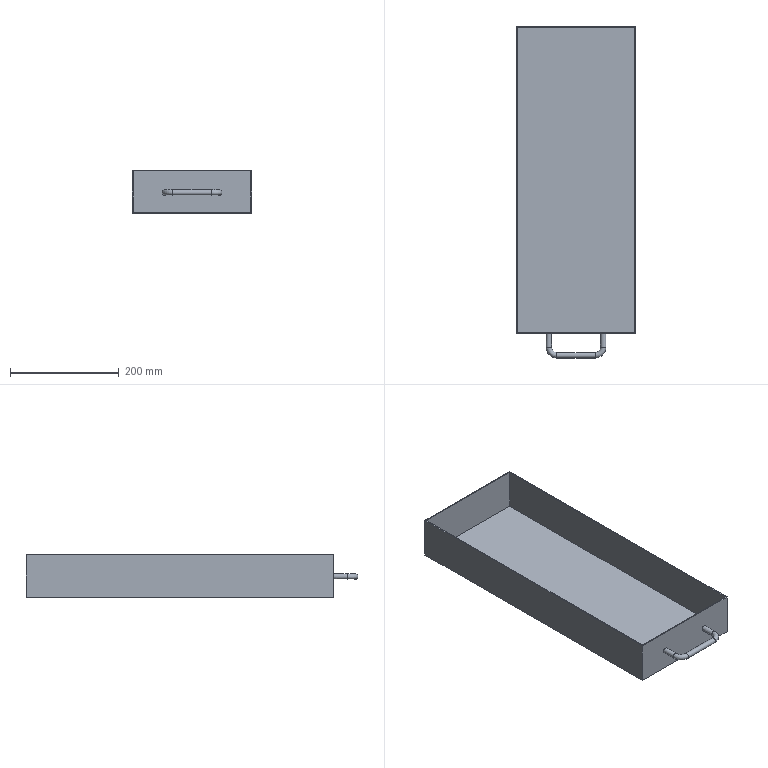Part | NX | features solid 2 | 1 solid | 16 faces | box 220 x 610 x 78 mm | volume 499150 mm3 | plane 11 | cylinder 3 | torus 2 | commonest cylinder face diameters 10 x3
STEP:
#1=CARTESIAN_POINT('',(425.,-410.,-285.));
#2=VERTEX_POINT('',#1);
#3=CARTESIAN_POINT('',(425.,-410.,-280.));
#4=DIRECTION('',(0.,-1.,0.));
#5=DIRECTION('',(0.,0.,-1.));
#6=AXIS2_PLACEMENT_3D('',#3,#4,#5);
#7=CIRCLE('',#6,5.);
#8=EDGE_CURVE('',#2,#2,#7,.T.);
#9=ORIENTED_EDGE('',*,*,#8,.F.);
#10=EDGE_LOOP('',(#9));
#11=FACE_BOUND('',#10,.T.);
#12=CARTESIAN_POINT('',(365.,-410.,-240.));
#13=VERTEX_POINT('',#12);
#14=CARTESIAN_POINT('',(585.,-410.,-240.));
#15=VERTEX_POINT('',#14);
#16=CARTESIAN_POINT('',(-350.,-410.,-240.));
#17=DIRECTION('',(1.,0.,0.));
#18=VECTOR('',#17,1000.);
#19=LINE('',#16,#18);
#20=EDGE_CURVE('',#13,#15,#19,.T.);
#21=ORIENTED_EDGE('',*,*,#20,.F.);
#22=CARTESIAN_POINT('',(365.,-410.,-318.));
#23=VERTEX_POINT('',#22);
#24=CARTESIAN_POINT('',(365.,-410.,0.));
#25=DIRECTION('',(0.,0.,1.));
#26=VECTOR('',#25,1000.);
#27=LINE('',#24,#26);
#28=EDGE_CURVE('',#23,#13,#27,.T.);
#29=ORIENTED_EDGE('',*,*,#28,.F.);
#30=CARTESIAN_POINT('',(585.,-410.,-318.));
#31=VERTEX_POINT('',#30);
#32=CARTESIAN_POINT('',(-350.,-410.,-318.));
#33=DIRECTION('',(-1.,0.,0.));
#34=VECTOR('',#33,1000.);
#35=LINE('',#32,#34);
#36=EDGE_CURVE('',#23,#31,#35,.F.);
#37=ORIENTED_EDGE('',*,*,#36,.T.);
#38=CARTESIAN_POINT('',(585.,-410.,0.));
#39=DIRECTION('',(0.,0.,1.));
#40=VECTOR('',#39,1000.);
#41=LINE('',#38,#40);
#42=EDGE_CURVE('',#31,#15,#41,.T.);
#43=ORIENTED_EDGE('',*,*,#42,.T.);
#44=EDGE_LOOP('',(#21,#29,#37,#43));
#45=FACE_BOUND('',#44,.T.);
#46=CARTESIAN_POINT('',(520.,-410.,-280.));
#47=VERTEX_POINT('',#46);
#48=CARTESIAN_POINT('',(525.,-410.,-280.));
#49=DIRECTION('',(0.,-1.,0.));
#50=DIRECTION('',(-1.,0.,0.));
#51=AXIS2_PLACEMENT_3D('',#48,#49,#50);
#52=CIRCLE('',#51,5.);
#53=EDGE_CURVE('',#47,#47,#52,.T.);
#54=ORIENTED_EDGE('',*,*,#53,.F.);
#55=EDGE_LOOP('',(#54));
#56=FACE_BOUND('',#55,.T.);
#57=CARTESIAN_POINT('',(360.,-410.,0.));
#58=DIRECTION('',(0.,-1.,0.));
#59=DIRECTION('',(0.,0.,-1.));
#60=AXIS2_PLACEMENT_3D('',#57,#58,#59);
#61=PLANE('',#60);
#62=ADVANCED_FACE('',(#11,#45,#56),#61,.T.);
#63=CARTESIAN_POINT('',(365.,155.,-240.));
#64=VERTEX_POINT('',#63);
#65=CARTESIAN_POINT('',(365.,105.,-240.));
#66=DIRECTION('',(0.,-1.,0.));
#67=VECTOR('',#66,1000.);
#68=LINE('',#65,#67);
#69=EDGE_CURVE('',#64,#13,#68,.T.);
#70=ORIENTED_EDGE('',*,*,#69,.F.);
#71=CARTESIAN_POINT('',(365.,155.,-318.));
#72=VERTEX_POINT('',#71);
#73=CARTESIAN_POINT('',(365.,155.,0.));
#74=DIRECTION('',(0.,0.,1.));
#75=VECTOR('',#74,1000.);
#76=LINE('',#73,#75);
#77=EDGE_CURVE('',#72,#64,#76,.T.);
#78=ORIENTED_EDGE('',*,*,#77,.F.);
#79=CARTESIAN_POINT('',(365.,-70.,-318.));
#80=DIRECTION('',(0.,1.,0.));
#81=VECTOR('',#80,1000.);
#82=LINE('',#79,#81);
#83=EDGE_CURVE('',#72,#23,#82,.F.);
#84=ORIENTED_EDGE('',*,*,#83,.T.);
#85=ORIENTED_EDGE('',*,*,#28,.T.);
#86=EDGE_LOOP('',(#70,#78,#84,#85));
#87=FACE_BOUND('',#86,.T.);
#88=CARTESIAN_POINT('',(365.,175.,0.));
#89=DIRECTION('',(-1.,0.,0.));
#90=DIRECTION('',(0.,0.,1.));
#91=AXIS2_PLACEMENT_3D('',#88,#89,#90);
#92=PLANE('',#91);
#93=ADVANCED_FACE('',(#87),#92,.T.);
#94=CARTESIAN_POINT('',(585.,155.,-240.));
#95=VERTEX_POINT('',#94);
#96=CARTESIAN_POINT('',(585.,105.,-240.));
#97=DIRECTION('',(0.,1.,0.));
#98=VECTOR('',#97,1000.);
#99=LINE('',#96,#98);
#100=EDGE_CURVE('',#15,#95,#99,.T.);
#101=ORIENTED_EDGE('',*,*,#100,.F.);
#102=ORIENTED_EDGE('',*,*,#42,.F.);
#103=CARTESIAN_POINT('',(585.,155.,-318.));
#104=VERTEX_POINT('',#103);
#105=CARTESIAN_POINT('',(585.,-70.,-318.));
#106=DIRECTION('',(0.,-1.,0.));
#107=VECTOR('',#106,1000.);
#108=LINE('',#105,#107);
#109=EDGE_CURVE('',#31,#104,#108,.F.);
#110=ORIENTED_EDGE('',*,*,#109,.T.);
#111=CARTESIAN_POINT('',(585.,155.,0.));
#112=DIRECTION('',(0.,0.,1.));
#113=VECTOR('',#112,1000.);
#114=LINE('',#111,#113);
#115=EDGE_CURVE('',#104,#95,#114,.T.);
#116=ORIENTED_EDGE('',*,*,#115,.T.);
#117=EDGE_LOOP('',(#101,#102,#110,#116));
#118=FACE_BOUND('',#117,.T.);
#119=CARTESIAN_POINT('',(585.,-460.,0.));
#120=DIRECTION('',(1.,0.,0.));
#121=DIRECTION('',(0.,0.,-1.));
#122=AXIS2_PLACEMENT_3D('',#119,#120,#121);
#123=PLANE('',#122);
#124=ADVANCED_FACE('',(#118),#123,.T.);
#125=CARTESIAN_POINT('',(-350.,155.,-240.));
#126=DIRECTION('',(-1.,0.,0.));
#127=VECTOR('',#126,1000.);
#128=LINE('',#125,#127);
#129=EDGE_CURVE('',#95,#64,#128,.T.);
#130=ORIENTED_EDGE('',*,*,#129,.F.);
#131=ORIENTED_EDGE('',*,*,#115,.F.);
#132=CARTESIAN_POINT('',(-350.,155.,-318.));
#133=DIRECTION('',(1.,0.,0.));
#134=VECTOR('',#133,1000.);
#135=LINE('',#132,#134);
#136=EDGE_CURVE('',#104,#72,#135,.F.);
#137=ORIENTED_EDGE('',*,*,#136,.T.);
#138=ORIENTED_EDGE('',*,*,#77,.T.);
#139=EDGE_LOOP('',(#130,#131,#137,#138));
#140=FACE_BOUND('',#139,.T.);
#141=CARTESIAN_POINT('',(585.,155.,0.));
#142=DIRECTION('',(0.,1.,0.));
#143=DIRECTION('',(0.,0.,1.));
#144=AXIS2_PLACEMENT_3D('',#141,#142,#143);
#145=PLANE('',#144);
#146=ADVANCED_FACE('',(#140),#145,.T.);
#147=ORIENTED_EDGE('',*,*,#83,.F.);
#148=ORIENTED_EDGE('',*,*,#136,.F.);
#149=ORIENTED_EDGE('',*,*,#109,.F.);
#150=ORIENTED_EDGE('',*,*,#36,.F.);
#151=EDGE_LOOP('',(#147,#148,#149,#150));
#152=FACE_BOUND('',#151,.T.);
#153=CARTESIAN_POINT('',(-350.,-70.,-318.));
#154=DIRECTION('',(0.,0.,-1.));
#155=DIRECTION('',(-1.,0.,0.));
#156=AXIS2_PLACEMENT_3D('',#153,#154,#155);
#157=PLANE('',#156);
#158=ADVANCED_FACE('',(#152),#157,.T.);
#159=CARTESIAN_POINT('',(367.,153.,-240.));
#160=VERTEX_POINT('',#159);
#161=CARTESIAN_POINT('',(367.,-408.,-240.));
#162=VERTEX_POINT('',#161);
#163=CARTESIAN_POINT('',(367.,105.,-240.));
#164=DIRECTION('',(0.,-1.,0.));
#165=VECTOR('',#164,1000.);
#166=LINE('',#163,#165);
#167=EDGE_CURVE('',#160,#162,#166,.T.);
#168=ORIENTED_EDGE('',*,*,#167,.F.);
#169=CARTESIAN_POINT('',(583.,153.,-240.));
#170=VERTEX_POINT('',#169);
#171=CARTESIAN_POINT('',(-350.,153.,-240.));
#172=DIRECTION('',(-1.,0.,0.));
#173=VECTOR('',#172,1000.);
#174=LINE('',#171,#173);
#175=EDGE_CURVE('',#170,#160,#174,.T.);
#176=ORIENTED_EDGE('',*,*,#175,.F.);
#177=CARTESIAN_POINT('',(583.,-408.,-240.));
#178=VERTEX_POINT('',#177);
#179=CARTESIAN_POINT('',(583.,105.,-240.));
#180=DIRECTION('',(0.,1.,0.));
#181=VECTOR('',#180,1000.);
#182=LINE('',#179,#181);
#183=EDGE_CURVE('',#178,#170,#182,.T.);
#184=ORIENTED_EDGE('',*,*,#183,.F.);
#185=CARTESIAN_POINT('',(-350.,-408.,-240.));
#186=DIRECTION('',(1.,0.,0.));
#187=VECTOR('',#186,1000.);
#188=LINE('',#185,#187);
#189=EDGE_CURVE('',#162,#178,#188,.T.);
#190=ORIENTED_EDGE('',*,*,#189,.F.);
#191=EDGE_LOOP('',(#168,#176,#184,#190));
#192=FACE_BOUND('',#191,.T.);
#193=ORIENTED_EDGE('',*,*,#69,.T.);
#194=ORIENTED_EDGE('',*,*,#20,.T.);
#195=ORIENTED_EDGE('',*,*,#100,.T.);
#196=ORIENTED_EDGE('',*,*,#129,.T.);
#197=EDGE_LOOP('',(#193,#194,#195,#196));
#198=FACE_BOUND('',#197,.T.);
#199=CARTESIAN_POINT('',(-350.,105.,-240.));
#200=DIRECTION('',(0.,0.,1.));
#201=DIRECTION('',(1.,0.,0.));
#202=AXIS2_PLACEMENT_3D('',#199,#200,#201);
#203=PLANE('',#202);
#204=ADVANCED_FACE('',(#192,#198),#203,.T.);
#205=ORIENTED_EDGE('',*,*,#167,.T.);
#206=CARTESIAN_POINT('',(367.,-408.,-316.));
#207=VERTEX_POINT('',#206);
#208=CARTESIAN_POINT('',(367.,-408.,0.));
#209=DIRECTION('',(0.,0.,1.));
#210=VECTOR('',#209,1000.);
#211=LINE('',#208,#210);
#212=EDGE_CURVE('',#207,#162,#211,.T.);
#213=ORIENTED_EDGE('',*,*,#212,.F.);
#214=CARTESIAN_POINT('',(367.,153.,-316.));
#215=VERTEX_POINT('',#214);
#216=CARTESIAN_POINT('',(367.,-70.,-316.));
#217=DIRECTION('',(0.,1.,0.));
#218=VECTOR('',#217,1000.);
#219=LINE('',#216,#218);
#220=EDGE_CURVE('',#215,#207,#219,.F.);
#221=ORIENTED_EDGE('',*,*,#220,.F.);
#222=CARTESIAN_POINT('',(367.,153.,0.));
#223=DIRECTION('',(0.,0.,1.));
#224=VECTOR('',#223,1000.);
#225=LINE('',#222,#224);
#226=EDGE_CURVE('',#215,#160,#225,.T.);
#227=ORIENTED_EDGE('',*,*,#226,.T.);
#228=EDGE_LOOP('',(#205,#213,#221,#227));
#229=FACE_BOUND('',#228,.T.);
#230=CARTESIAN_POINT('',(367.,175.,0.));
#231=DIRECTION('',(-1.,0.,0.));
#232=DIRECTION('',(0.,0.,1.));
#233=AXIS2_PLACEMENT_3D('',#230,#231,#232);
#234=PLANE('',#233);
#235=ADVANCED_FACE('',(#229),#234,.F.);
#236=ORIENTED_EDGE('',*,*,#189,.T.);
#237=CARTESIAN_POINT('',(583.,-408.,-316.));
#238=VERTEX_POINT('',#237);
#239=CARTESIAN_POINT('',(583.,-408.,0.));
#240=DIRECTION('',(0.,0.,1.));
#241=VECTOR('',#240,1000.);
#242=LINE('',#239,#241);
#243=EDGE_CURVE('',#238,#178,#242,.T.);
#244=ORIENTED_EDGE('',*,*,#243,.F.);
#245=CARTESIAN_POINT('',(-350.,-408.,-316.));
#246=DIRECTION('',(-1.,0.,0.));
#247=VECTOR('',#246,1000.);
#248=LINE('',#245,#247);
#249=EDGE_CURVE('',#207,#238,#248,.F.);
#250=ORIENTED_EDGE('',*,*,#249,.F.);
#251=ORIENTED_EDGE('',*,*,#212,.T.);
#252=EDGE_LOOP('',(#236,#244,#250,#251));
#253=FACE_BOUND('',#252,.T.);
#254=CARTESIAN_POINT('',(360.,-408.,0.));
#255=DIRECTION('',(0.,-1.,0.));
#256=DIRECTION('',(0.,0.,-1.));
#257=AXIS2_PLACEMENT_3D('',#254,#255,#256);
#258=PLANE('',#257);
#259=ADVANCED_FACE('',(#253),#258,.F.);
#260=ORIENTED_EDGE('',*,*,#183,.T.);
#261=CARTESIAN_POINT('',(583.,153.,-316.));
#262=VERTEX_POINT('',#261);
#263=CARTESIAN_POINT('',(583.,153.,0.));
#264=DIRECTION('',(0.,0.,1.));
#265=VECTOR('',#264,1000.);
#266=LINE('',#263,#265);
#267=EDGE_CURVE('',#262,#170,#266,.T.);
#268=ORIENTED_EDGE('',*,*,#267,.F.);
#269=CARTESIAN_POINT('',(583.,-70.,-316.));
#270=DIRECTION('',(0.,-1.,0.));
#271=VECTOR('',#270,1000.);
#272=LINE('',#269,#271);
#273=EDGE_CURVE('',#238,#262,#272,.F.);
#274=ORIENTED_EDGE('',*,*,#273,.F.);
#275=ORIENTED_EDGE('',*,*,#243,.T.);
#276=EDGE_LOOP('',(#260,#268,#274,#275));
#277=FACE_BOUND('',#276,.T.);
#278=CARTESIAN_POINT('',(583.,-460.,0.));
#279=DIRECTION('',(1.,0.,0.));
#280=DIRECTION('',(0.,0.,-1.));
#281=AXIS2_PLACEMENT_3D('',#278,#279,#280);
#282=PLANE('',#281);
#283=ADVANCED_FACE('',(#277),#282,.F.);
#284=ORIENTED_EDGE('',*,*,#175,.T.);
#285=ORIENTED_EDGE('',*,*,#226,.F.);
#286=CARTESIAN_POINT('',(-350.,153.,-316.));
#287=DIRECTION('',(1.,0.,0.));
#288=VECTOR('',#287,1000.);
#289=LINE('',#286,#288);
#290=EDGE_CURVE('',#262,#215,#289,.F.);
#291=ORIENTED_EDGE('',*,*,#290,.F.);
#292=ORIENTED_EDGE('',*,*,#267,.T.);
#293=EDGE_LOOP('',(#284,#285,#291,#292));
#294=FACE_BOUND('',#293,.T.);
#295=CARTESIAN_POINT('',(585.,153.,0.));
#296=DIRECTION('',(0.,1.,0.));
#297=DIRECTION('',(0.,0.,1.));
#298=AXIS2_PLACEMENT_3D('',#295,#296,#297);
#299=PLANE('',#298);
#300=ADVANCED_FACE('',(#294),#299,.F.);
#301=ORIENTED_EDGE('',*,*,#220,.T.);
#302=ORIENTED_EDGE('',*,*,#249,.T.);
#303=ORIENTED_EDGE('',*,*,#273,.T.);
#304=ORIENTED_EDGE('',*,*,#290,.T.);
#305=EDGE_LOOP('',(#301,#302,#303,#304));
#306=FACE_BOUND('',#305,.T.);
#307=CARTESIAN_POINT('',(-350.,-70.,-316.));
#308=DIRECTION('',(0.,0.,-1.));
#309=DIRECTION('',(-1.,0.,0.));
#310=AXIS2_PLACEMENT_3D('',#307,#308,#309);
#311=PLANE('',#310);
#312=ADVANCED_FACE('',(#306),#311,.F.);
#313=CARTESIAN_POINT('',(520.,-435.,-280.));
#314=VERTEX_POINT('',#313);
#315=CARTESIAN_POINT('',(525.,-435.,-280.));
#316=DIRECTION('',(0.,-1.,0.));
#317=DIRECTION('',(-1.,0.,0.));
#318=AXIS2_PLACEMENT_3D('',#315,#316,#317);
#319=CIRCLE('',#318,5.);
#320=EDGE_CURVE('',#314,#314,#319,.T.);
#321=ORIENTED_EDGE('',*,*,#320,.F.);
#322=EDGE_LOOP('',(#321));
#323=FACE_BOUND('',#322,.T.);
#324=ORIENTED_EDGE('',*,*,#53,.T.);
#325=EDGE_LOOP('',(#324));
#326=FACE_BOUND('',#325,.T.);
#327=CARTESIAN_POINT('',(525.,-435.,-280.));
#328=DIRECTION('',(0.,1.,0.));
#329=DIRECTION('',(0.,0.,1.));
#330=AXIS2_PLACEMENT_3D('',#327,#328,#329);
#331=CYLINDRICAL_SURFACE('',#330,5.);
#332=ADVANCED_FACE('',(#323,#326),#331,.T.);
#333=CARTESIAN_POINT('',(510.,-445.,-280.));
#334=VERTEX_POINT('',#333);
#335=CARTESIAN_POINT('',(510.,-450.,-280.));
#336=DIRECTION('',(-1.,0.,0.));
#337=DIRECTION('',(0.,1.,0.));
#338=AXIS2_PLACEMENT_3D('',#335,#336,#337);
#339=CIRCLE('',#338,5.);
#340=EDGE_CURVE('',#334,#334,#339,.T.);
#341=ORIENTED_EDGE('',*,*,#340,.F.);
#342=EDGE_LOOP('',(#341));
#343=FACE_BOUND('',#342,.T.);
#344=ORIENTED_EDGE('',*,*,#320,.T.);
#345=EDGE_LOOP('',(#344));
#346=FACE_BOUND('',#345,.T.);
#347=CARTESIAN_POINT('',(510.,-435.,-280.));
#348=DIRECTION('',(0.,0.,1.));
#349=DIRECTION('',(1.,0.,0.));
#350=AXIS2_PLACEMENT_3D('',#347,#348,#349);
#351=TOROIDAL_SURFACE('',#350,15.,5.);
#352=ADVANCED_FACE('',(#343,#346),#351,.T.);
#353=ORIENTED_EDGE('',*,*,#340,.T.);
#354=EDGE_LOOP('',(#353));
#355=FACE_BOUND('',#354,.T.);
#356=CARTESIAN_POINT('',(440.,-445.,-280.));
#357=VERTEX_POINT('',#356);
#358=CARTESIAN_POINT('',(440.,-450.,-280.));
#359=DIRECTION('',(-1.,0.,0.));
#360=DIRECTION('',(0.,1.,0.));
#361=AXIS2_PLACEMENT_3D('',#358,#359,#360);
#362=CIRCLE('',#361,5.);
#363=EDGE_CURVE('',#357,#357,#362,.T.);
#364=ORIENTED_EDGE('',*,*,#363,.F.);
#365=EDGE_LOOP('',(#364));
#366=FACE_BOUND('',#365,.T.);
#367=CARTESIAN_POINT('',(440.,-450.,-280.));
#368=DIRECTION('',(1.,0.,0.));
#369=DIRECTION('',(0.,0.,-1.));
#370=AXIS2_PLACEMENT_3D('',#367,#368,#369);
#371=CYLINDRICAL_SURFACE('',#370,5.);
#372=ADVANCED_FACE('',(#355,#366),#371,.T.);
#373=CARTESIAN_POINT('',(430.,-435.,-280.));
#374=VERTEX_POINT('',#373);
#375=CARTESIAN_POINT('',(425.,-435.,-280.));
#376=DIRECTION('',(0.,1.,0.));
#377=DIRECTION('',(1.,0.,0.));
#378=AXIS2_PLACEMENT_3D('',#375,#376,#377);
#379=CIRCLE('',#378,5.);
#380=EDGE_CURVE('',#374,#374,#379,.T.);
#381=ORIENTED_EDGE('',*,*,#380,.F.);
#382=EDGE_LOOP('',(#381));
#383=FACE_BOUND('',#382,.T.);
#384=ORIENTED_EDGE('',*,*,#363,.T.);
#385=EDGE_LOOP('',(#384));
#386=FACE_BOUND('',#385,.T.);
#387=CARTESIAN_POINT('',(440.,-435.,-280.));
#388=DIRECTION('',(0.,0.,1.));
#389=DIRECTION('',(1.,0.,0.));
#390=AXIS2_PLACEMENT_3D('',#387,#388,#389);
#391=TOROIDAL_SURFACE('',#390,15.,5.);
#392=ADVANCED_FACE('',(#383,#386),#391,.T.);
#393=ORIENTED_EDGE('',*,*,#380,.T.);
#394=EDGE_LOOP('',(#393));
#395=FACE_BOUND('',#394,.T.);
#396=ORIENTED_EDGE('',*,*,#8,.T.);
#397=EDGE_LOOP('',(#396));
#398=FACE_BOUND('',#397,.T.);
#399=CARTESIAN_POINT('',(425.,-435.,-280.));
#400=DIRECTION('',(0.,1.,0.));
#401=DIRECTION('',(0.,0.,1.));
#402=AXIS2_PLACEMENT_3D('',#399,#400,#401);
#403=CYLINDRICAL_SURFACE('',#402,5.);
#404=ADVANCED_FACE('',(#395,#398),#403,.T.);
#405=CLOSED_SHELL('',(#62,#93,#124,#146,#158,#204,#235,#259,#283,#300,#312,#332,#352,#372,#392,#404));
#406=MANIFOLD_SOLID_BREP('',#405);
#407=(LENGTH_UNIT()NAMED_UNIT(*)SI_UNIT(.MILLI.,.METRE.));
#408=UNCERTAINTY_MEASURE_WITH_UNIT(LENGTH_MEASURE(0.00001),#407,'','');
#409=(NAMED_UNIT(*)PLANE_ANGLE_UNIT()SI_UNIT($,.RADIAN.));
#410=(NAMED_UNIT(*)SI_UNIT($,.STERADIAN.)SOLID_ANGLE_UNIT());
#411=(GEOMETRIC_REPRESENTATION_CONTEXT(3)GLOBAL_UNCERTAINTY_ASSIGNED_CONTEXT((#408))GLOBAL_UNIT_ASSIGNED_CONTEXT((#407,#409,#410))REPRESENTATION_CONTEXT('',''));
#412=ADVANCED_BREP_SHAPE_REPRESENTATION('',(#406),#411);